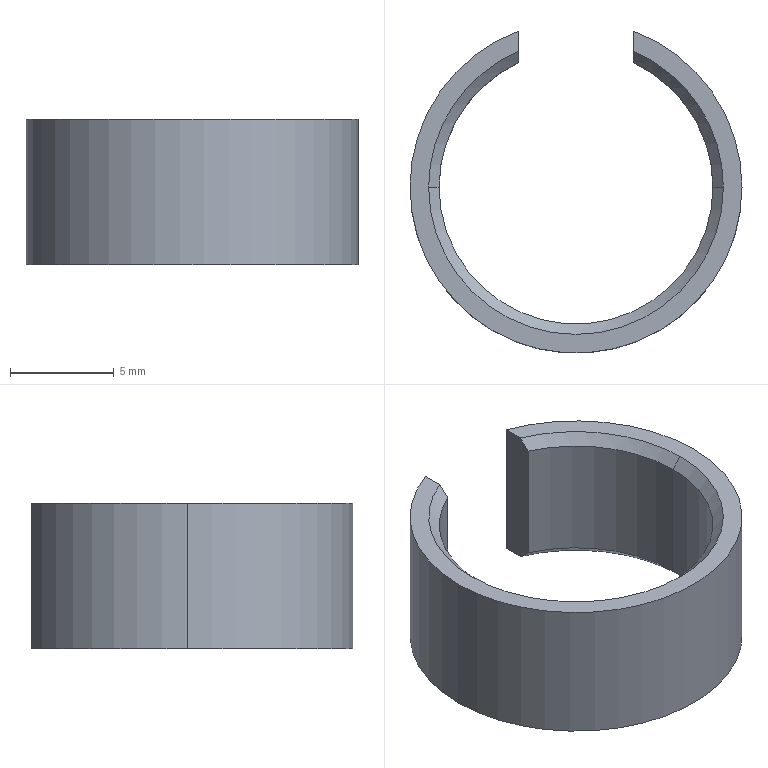Part | SolidWorks | features Chamfer 1, Extrusion 1, ICE 1 | 1 solid | 16 faces | box 16 x 15.512 x 7 mm | volume 385.007 mm3 | cone 6 | cylinder 6 | plane 4 | commonest cylinder face diameters 13.2 x3 16 x3
STEP:
#1=CARTESIAN_POINT('',(-6.6,0.,6.5));
#2=VERTEX_POINT('',#1);
#3=CARTESIAN_POINT('',(6.6,0.,6.5));
#4=VERTEX_POINT('',#3);
#5=CARTESIAN_POINT('',(0.,0.,6.5));
#6=DIRECTION('',(0.,0.,1.));
#7=DIRECTION('',(1.,0.,0.));
#8=AXIS2_PLACEMENT_3D('',#5,#6,#7);
#9=CIRCLE('',#8,6.6);
#10=EDGE_CURVE('',#2,#4,#9,.T.);
#11=ORIENTED_EDGE('',*,*,#10,.F.);
#12=CARTESIAN_POINT('',(-7.1,0.,7.));
#13=VERTEX_POINT('',#12);
#14=CARTESIAN_POINT('',(-6.6,0.,6.5));
#15=DIRECTION('',(-0.7071,0.,0.7071));
#16=VECTOR('',#15,1000.);
#17=LINE('',#14,#16);
#18=EDGE_CURVE('',#2,#13,#17,.T.);
#19=ORIENTED_EDGE('',*,*,#18,.T.);
#20=CARTESIAN_POINT('',(7.1,0.,7.));
#21=VERTEX_POINT('',#20);
#22=CARTESIAN_POINT('',(0.,0.,7.));
#23=DIRECTION('',(0.,0.,-1.));
#24=DIRECTION('',(1.,0.,0.));
#25=AXIS2_PLACEMENT_3D('',#22,#23,#24);
#26=CIRCLE('',#25,7.1);
#27=EDGE_CURVE('',#21,#13,#26,.T.);
#28=ORIENTED_EDGE('',*,*,#27,.F.);
#29=CARTESIAN_POINT('',(6.6,0.,6.5));
#30=DIRECTION('',(0.7071,0.,0.7071));
#31=VECTOR('',#30,1000.);
#32=LINE('',#29,#31);
#33=EDGE_CURVE('',#4,#21,#32,.T.);
#34=ORIENTED_EDGE('',*,*,#33,.F.);
#35=EDGE_LOOP('',(#11,#19,#28,#34));
#36=FACE_OUTER_BOUND('',#35,.T.);
#37=CARTESIAN_POINT('',(0.,0.,6.5));
#38=DIRECTION('',(0.,0.,1.));
#39=DIRECTION('',(1.,0.,0.));
#40=AXIS2_PLACEMENT_3D('',#37,#38,#39);
#41=CONICAL_SURFACE('',#40,6.6,0.7854);
#42=ADVANCED_FACE('',(#36),#41,.F.);
#43=CARTESIAN_POINT('',(2.75,6.,6.5));
#44=VERTEX_POINT('',#43);
#45=CARTESIAN_POINT('',(0.,0.,6.5));
#46=DIRECTION('',(0.,0.,1.));
#47=DIRECTION('',(1.,0.,0.));
#48=AXIS2_PLACEMENT_3D('',#45,#46,#47);
#49=CIRCLE('',#48,6.6);
#50=EDGE_CURVE('',#4,#44,#49,.T.);
#51=ORIENTED_EDGE('',*,*,#50,.F.);
#52=ORIENTED_EDGE('',*,*,#33,.T.);
#53=CARTESIAN_POINT('',(2.75,6.546,7.));
#54=VERTEX_POINT('',#53);
#55=CARTESIAN_POINT('',(0.,0.,7.));
#56=DIRECTION('',(0.,0.,-1.));
#57=DIRECTION('',(1.,0.,0.));
#58=AXIS2_PLACEMENT_3D('',#55,#56,#57);
#59=CIRCLE('',#58,7.1);
#60=EDGE_CURVE('',#54,#21,#59,.T.);
#61=ORIENTED_EDGE('',*,*,#60,.F.);
#62=CARTESIAN_POINT('',(2.75,6.,6.5));
#63=CARTESIAN_POINT('',(2.75,6.182,6.666));
#64=CARTESIAN_POINT('',(2.75,6.364,6.833));
#65=CARTESIAN_POINT('',(2.75,6.546,7.));
#66=B_SPLINE_CURVE_WITH_KNOTS('',3,(#62,#63,#64,#65),.UNSPECIFIED.,.F.,.F.,(4,4),(0.,0.0007404),.UNSPECIFIED.);
#67=EDGE_CURVE('',#44,#54,#66,.T.);
#68=ORIENTED_EDGE('',*,*,#67,.F.);
#69=EDGE_LOOP('',(#51,#52,#61,#68));
#70=FACE_OUTER_BOUND('',#69,.T.);
#71=CARTESIAN_POINT('',(0.,0.,6.5));
#72=DIRECTION('',(0.,0.,1.));
#73=DIRECTION('',(1.,0.,0.));
#74=AXIS2_PLACEMENT_3D('',#71,#72,#73);
#75=CONICAL_SURFACE('',#74,6.6,0.7854);
#76=ADVANCED_FACE('',(#70),#75,.F.);
#77=CARTESIAN_POINT('',(6.6,0.,0.5));
#78=VERTEX_POINT('',#77);
#79=CARTESIAN_POINT('',(-6.6,0.,0.5));
#80=VERTEX_POINT('',#79);
#81=CARTESIAN_POINT('',(0.,0.,0.5));
#82=DIRECTION('',(0.,0.,-1.));
#83=DIRECTION('',(1.,0.,0.));
#84=AXIS2_PLACEMENT_3D('',#81,#82,#83);
#85=CIRCLE('',#84,6.6);
#86=EDGE_CURVE('',#78,#80,#85,.T.);
#87=ORIENTED_EDGE('',*,*,#86,.F.);
#88=CARTESIAN_POINT('',(7.1,0.,0.));
#89=VERTEX_POINT('',#88);
#90=CARTESIAN_POINT('',(7.1,0.,0.));
#91=DIRECTION('',(0.7071,0.,-0.7071));
#92=VECTOR('',#91,1000.);
#93=LINE('',#90,#92);
#94=EDGE_CURVE('',#78,#89,#93,.T.);
#95=ORIENTED_EDGE('',*,*,#94,.T.);
#96=CARTESIAN_POINT('',(-7.1,0.,0.));
#97=VERTEX_POINT('',#96);
#98=CARTESIAN_POINT('',(0.,0.,0.));
#99=DIRECTION('',(0.,0.,1.));
#100=DIRECTION('',(1.,0.,0.));
#101=AXIS2_PLACEMENT_3D('',#98,#99,#100);
#102=CIRCLE('',#101,7.1);
#103=EDGE_CURVE('',#97,#89,#102,.T.);
#104=ORIENTED_EDGE('',*,*,#103,.F.);
#105=CARTESIAN_POINT('',(-7.1,0.,0.));
#106=DIRECTION('',(-0.7071,0.,-0.7071));
#107=VECTOR('',#106,1000.);
#108=LINE('',#105,#107);
#109=EDGE_CURVE('',#80,#97,#108,.T.);
#110=ORIENTED_EDGE('',*,*,#109,.F.);
#111=EDGE_LOOP('',(#87,#95,#104,#110));
#112=FACE_OUTER_BOUND('',#111,.T.);
#113=CARTESIAN_POINT('',(0.,0.,0.));
#114=DIRECTION('',(0.,0.,-1.));
#115=DIRECTION('',(-1.,0.,0.));
#116=AXIS2_PLACEMENT_3D('',#113,#114,#115);
#117=CONICAL_SURFACE('',#116,7.1,0.7854);
#118=ADVANCED_FACE('',(#112),#117,.F.);
#119=CARTESIAN_POINT('',(-2.75,6.,0.5));
#120=VERTEX_POINT('',#119);
#121=CARTESIAN_POINT('',(0.,0.,0.5));
#122=DIRECTION('',(0.,0.,-1.));
#123=DIRECTION('',(1.,0.,0.));
#124=AXIS2_PLACEMENT_3D('',#121,#122,#123);
#125=CIRCLE('',#124,6.6);
#126=EDGE_CURVE('',#80,#120,#125,.T.);
#127=ORIENTED_EDGE('',*,*,#126,.F.);
#128=ORIENTED_EDGE('',*,*,#109,.T.);
#129=CARTESIAN_POINT('',(-2.75,6.546,0.));
#130=VERTEX_POINT('',#129);
#131=CARTESIAN_POINT('',(0.,0.,0.));
#132=DIRECTION('',(0.,0.,1.));
#133=DIRECTION('',(1.,0.,0.));
#134=AXIS2_PLACEMENT_3D('',#131,#132,#133);
#135=CIRCLE('',#134,7.1);
#136=EDGE_CURVE('',#130,#97,#135,.T.);
#137=ORIENTED_EDGE('',*,*,#136,.F.);
#138=CARTESIAN_POINT('',(-2.75,6.,0.5));
#139=CARTESIAN_POINT('',(-2.75,6.182,0.334));
#140=CARTESIAN_POINT('',(-2.75,6.364,0.1673));
#141=CARTESIAN_POINT('',(-2.75,6.546,0.));
#142=B_SPLINE_CURVE_WITH_KNOTS('',3,(#138,#139,#140,#141),.UNSPECIFIED.,.F.,.F.,(4,4),(0.,0.0007404),.UNSPECIFIED.);
#143=EDGE_CURVE('',#120,#130,#142,.T.);
#144=ORIENTED_EDGE('',*,*,#143,.F.);
#145=EDGE_LOOP('',(#127,#128,#137,#144));
#146=FACE_OUTER_BOUND('',#145,.T.);
#147=CARTESIAN_POINT('',(0.,0.,0.));
#148=DIRECTION('',(0.,0.,-1.));
#149=DIRECTION('',(-1.,0.,0.));
#150=AXIS2_PLACEMENT_3D('',#147,#148,#149);
#151=CONICAL_SURFACE('',#150,7.1,0.7854);
#152=ADVANCED_FACE('',(#146),#151,.F.);
#153=ORIENTED_EDGE('',*,*,#10,.T.);
#154=CARTESIAN_POINT('',(6.6,0.,7.));
#155=DIRECTION('',(0.,0.,-1.));
#156=VECTOR('',#155,1000.);
#157=LINE('',#154,#156);
#158=EDGE_CURVE('',#4,#78,#157,.T.);
#159=ORIENTED_EDGE('',*,*,#158,.T.);
#160=ORIENTED_EDGE('',*,*,#86,.T.);
#161=CARTESIAN_POINT('',(-6.6,0.,7.));
#162=DIRECTION('',(0.,0.,-1.));
#163=VECTOR('',#162,1000.);
#164=LINE('',#161,#163);
#165=EDGE_CURVE('',#2,#80,#164,.T.);
#166=ORIENTED_EDGE('',*,*,#165,.F.);
#167=EDGE_LOOP('',(#153,#159,#160,#166));
#168=FACE_OUTER_BOUND('',#167,.T.);
#169=CARTESIAN_POINT('',(0.,0.,7.));
#170=DIRECTION('',(0.,0.,-1.));
#171=DIRECTION('',(-1.,0.,0.));
#172=AXIS2_PLACEMENT_3D('',#169,#170,#171);
#173=CYLINDRICAL_SURFACE('',#172,6.6);
#174=ADVANCED_FACE('',(#168),#173,.F.);
#175=CARTESIAN_POINT('',(-2.75,6.,6.5));
#176=VERTEX_POINT('',#175);
#177=CARTESIAN_POINT('',(0.,0.,6.5));
#178=DIRECTION('',(0.,0.,1.));
#179=DIRECTION('',(1.,0.,0.));
#180=AXIS2_PLACEMENT_3D('',#177,#178,#179);
#181=CIRCLE('',#180,6.6);
#182=EDGE_CURVE('',#176,#2,#181,.T.);
#183=ORIENTED_EDGE('',*,*,#182,.T.);
#184=ORIENTED_EDGE('',*,*,#165,.T.);
#185=ORIENTED_EDGE('',*,*,#126,.T.);
#186=CARTESIAN_POINT('',(-2.75,6.,7.));
#187=DIRECTION('',(0.,0.,-1.));
#188=VECTOR('',#187,1000.);
#189=LINE('',#186,#188);
#190=EDGE_CURVE('',#176,#120,#189,.T.);
#191=ORIENTED_EDGE('',*,*,#190,.F.);
#192=EDGE_LOOP('',(#183,#184,#185,#191));
#193=FACE_OUTER_BOUND('',#192,.T.);
#194=CARTESIAN_POINT('',(0.,0.,7.));
#195=DIRECTION('',(0.,0.,-1.));
#196=DIRECTION('',(-1.,0.,0.));
#197=AXIS2_PLACEMENT_3D('',#194,#195,#196);
#198=CYLINDRICAL_SURFACE('',#197,6.6);
#199=ADVANCED_FACE('',(#193),#198,.F.);
#200=CARTESIAN_POINT('',(8.,0.,7.));
#201=VERTEX_POINT('',#200);
#202=CARTESIAN_POINT('',(2.75,7.512,7.));
#203=VERTEX_POINT('',#202);
#204=CARTESIAN_POINT('',(0.,0.,7.));
#205=DIRECTION('',(0.,0.,1.));
#206=DIRECTION('',(1.,0.,0.));
#207=AXIS2_PLACEMENT_3D('',#204,#205,#206);
#208=CIRCLE('',#207,8.);
#209=EDGE_CURVE('',#201,#203,#208,.T.);
#210=ORIENTED_EDGE('',*,*,#209,.F.);
#211=CARTESIAN_POINT('',(8.,0.,0.));
#212=VERTEX_POINT('',#211);
#213=CARTESIAN_POINT('',(8.,0.,7.));
#214=DIRECTION('',(0.,0.,-1.));
#215=VECTOR('',#214,1000.);
#216=LINE('',#213,#215);
#217=EDGE_CURVE('',#201,#212,#216,.T.);
#218=ORIENTED_EDGE('',*,*,#217,.T.);
#219=CARTESIAN_POINT('',(2.75,7.512,0.));
#220=VERTEX_POINT('',#219);
#221=CARTESIAN_POINT('',(0.,0.,0.));
#222=DIRECTION('',(0.,0.,1.));
#223=DIRECTION('',(1.,0.,0.));
#224=AXIS2_PLACEMENT_3D('',#221,#222,#223);
#225=CIRCLE('',#224,8.);
#226=EDGE_CURVE('',#212,#220,#225,.T.);
#227=ORIENTED_EDGE('',*,*,#226,.T.);
#228=CARTESIAN_POINT('',(2.75,7.512,7.));
#229=DIRECTION('',(0.,0.,1.));
#230=VECTOR('',#229,1000.);
#231=LINE('',#228,#230);
#232=EDGE_CURVE('',#220,#203,#231,.T.);
#233=ORIENTED_EDGE('',*,*,#232,.T.);
#234=EDGE_LOOP('',(#210,#218,#227,#233));
#235=FACE_OUTER_BOUND('',#234,.T.);
#236=CARTESIAN_POINT('',(0.,0.,7.));
#237=DIRECTION('',(0.,0.,-1.));
#238=DIRECTION('',(-1.,0.,0.));
#239=AXIS2_PLACEMENT_3D('',#236,#237,#238);
#240=CYLINDRICAL_SURFACE('',#239,8.);
#241=ADVANCED_FACE('',(#235),#240,.T.);
#242=ORIENTED_EDGE('',*,*,#217,.F.);
#243=CARTESIAN_POINT('',(-8.,0.,7.));
#244=VERTEX_POINT('',#243);
#245=CARTESIAN_POINT('',(0.,0.,7.));
#246=DIRECTION('',(0.,0.,1.));
#247=DIRECTION('',(1.,0.,0.));
#248=AXIS2_PLACEMENT_3D('',#245,#246,#247);
#249=CIRCLE('',#248,8.);
#250=EDGE_CURVE('',#244,#201,#249,.T.);
#251=ORIENTED_EDGE('',*,*,#250,.F.);
#252=CARTESIAN_POINT('',(-8.,0.,0.));
#253=VERTEX_POINT('',#252);
#254=CARTESIAN_POINT('',(-8.,0.,7.));
#255=DIRECTION('',(0.,0.,-1.));
#256=VECTOR('',#255,1000.);
#257=LINE('',#254,#256);
#258=EDGE_CURVE('',#244,#253,#257,.T.);
#259=ORIENTED_EDGE('',*,*,#258,.T.);
#260=CARTESIAN_POINT('',(0.,0.,0.));
#261=DIRECTION('',(0.,0.,1.));
#262=DIRECTION('',(1.,0.,0.));
#263=AXIS2_PLACEMENT_3D('',#260,#261,#262);
#264=CIRCLE('',#263,8.);
#265=EDGE_CURVE('',#253,#212,#264,.T.);
#266=ORIENTED_EDGE('',*,*,#265,.T.);
#267=EDGE_LOOP('',(#242,#251,#259,#266));
#268=FACE_OUTER_BOUND('',#267,.T.);
#269=CARTESIAN_POINT('',(0.,0.,7.));
#270=DIRECTION('',(0.,0.,-1.));
#271=DIRECTION('',(-1.,0.,0.));
#272=AXIS2_PLACEMENT_3D('',#269,#270,#271);
#273=CYLINDRICAL_SURFACE('',#272,8.);
#274=ADVANCED_FACE('',(#268),#273,.T.);
#275=CARTESIAN_POINT('',(2.75,3.871,7.));
#276=DIRECTION('',(0.,1.,0.));
#277=VECTOR('',#276,1000.);
#278=LINE('',#275,#277);
#279=EDGE_CURVE('',#54,#203,#278,.T.);
#280=ORIENTED_EDGE('',*,*,#279,.F.);
#281=ORIENTED_EDGE('',*,*,#60,.T.);
#282=ORIENTED_EDGE('',*,*,#27,.T.);
#283=CARTESIAN_POINT('',(-2.75,6.546,7.));
#284=VERTEX_POINT('',#283);
#285=CARTESIAN_POINT('',(0.,0.,7.));
#286=DIRECTION('',(0.,0.,-1.));
#287=DIRECTION('',(1.,0.,0.));
#288=AXIS2_PLACEMENT_3D('',#285,#286,#287);
#289=CIRCLE('',#288,7.1);
#290=EDGE_CURVE('',#13,#284,#289,.T.);
#291=ORIENTED_EDGE('',*,*,#290,.T.);
#292=CARTESIAN_POINT('',(-2.75,7.512,7.));
#293=VERTEX_POINT('',#292);
#294=CARTESIAN_POINT('',(-2.75,3.871,7.));
#295=DIRECTION('',(0.,-1.,0.));
#296=VECTOR('',#295,1000.);
#297=LINE('',#294,#296);
#298=EDGE_CURVE('',#293,#284,#297,.T.);
#299=ORIENTED_EDGE('',*,*,#298,.F.);
#300=CARTESIAN_POINT('',(0.,0.,7.));
#301=DIRECTION('',(0.,0.,1.));
#302=DIRECTION('',(1.,0.,0.));
#303=AXIS2_PLACEMENT_3D('',#300,#301,#302);
#304=CIRCLE('',#303,8.);
#305=EDGE_CURVE('',#293,#244,#304,.T.);
#306=ORIENTED_EDGE('',*,*,#305,.T.);
#307=ORIENTED_EDGE('',*,*,#250,.T.);
#308=ORIENTED_EDGE('',*,*,#209,.T.);
#309=EDGE_LOOP('',(#280,#281,#282,#291,#299,#306,#307,#308));
#310=FACE_OUTER_BOUND('',#309,.T.);
#311=CARTESIAN_POINT('',(0.,0.,7.));
#312=DIRECTION('',(0.,0.,1.));
#313=DIRECTION('',(1.,0.,0.));
#314=AXIS2_PLACEMENT_3D('',#311,#312,#313);
#315=PLANE('',#314);
#316=ADVANCED_FACE('',(#310),#315,.T.);
#317=CARTESIAN_POINT('',(-2.75,7.512,0.));
#318=VERTEX_POINT('',#317);
#319=CARTESIAN_POINT('',(-2.75,3.871,0.));
#320=DIRECTION('',(0.,-1.,0.));
#321=VECTOR('',#320,1000.);
#322=LINE('',#319,#321);
#323=EDGE_CURVE('',#318,#130,#322,.T.);
#324=ORIENTED_EDGE('',*,*,#323,.T.);
#325=ORIENTED_EDGE('',*,*,#136,.T.);
#326=ORIENTED_EDGE('',*,*,#103,.T.);
#327=CARTESIAN_POINT('',(2.75,6.546,0.));
#328=VERTEX_POINT('',#327);
#329=CARTESIAN_POINT('',(0.,0.,0.));
#330=DIRECTION('',(0.,0.,1.));
#331=DIRECTION('',(1.,0.,0.));
#332=AXIS2_PLACEMENT_3D('',#329,#330,#331);
#333=CIRCLE('',#332,7.1);
#334=EDGE_CURVE('',#89,#328,#333,.T.);
#335=ORIENTED_EDGE('',*,*,#334,.T.);
#336=CARTESIAN_POINT('',(2.75,3.871,0.));
#337=DIRECTION('',(0.,1.,0.));
#338=VECTOR('',#337,1000.);
#339=LINE('',#336,#338);
#340=EDGE_CURVE('',#328,#220,#339,.T.);
#341=ORIENTED_EDGE('',*,*,#340,.T.);
#342=ORIENTED_EDGE('',*,*,#226,.F.);
#343=ORIENTED_EDGE('',*,*,#265,.F.);
#344=CARTESIAN_POINT('',(0.,0.,0.));
#345=DIRECTION('',(0.,0.,1.));
#346=DIRECTION('',(1.,0.,0.));
#347=AXIS2_PLACEMENT_3D('',#344,#345,#346);
#348=CIRCLE('',#347,8.);
#349=EDGE_CURVE('',#318,#253,#348,.T.);
#350=ORIENTED_EDGE('',*,*,#349,.F.);
#351=EDGE_LOOP('',(#324,#325,#326,#335,#341,#342,#343,#350));
#352=FACE_OUTER_BOUND('',#351,.T.);
#353=CARTESIAN_POINT('',(0.,0.,0.));
#354=DIRECTION('',(0.,0.,1.));
#355=DIRECTION('',(1.,0.,0.));
#356=AXIS2_PLACEMENT_3D('',#353,#354,#355);
#357=PLANE('',#356);
#358=ADVANCED_FACE('',(#352),#357,.F.);
#359=ORIENTED_EDGE('',*,*,#258,.F.);
#360=ORIENTED_EDGE('',*,*,#305,.F.);
#361=CARTESIAN_POINT('',(-2.75,7.512,7.));
#362=DIRECTION('',(0.,0.,-1.));
#363=VECTOR('',#362,1000.);
#364=LINE('',#361,#363);
#365=EDGE_CURVE('',#293,#318,#364,.T.);
#366=ORIENTED_EDGE('',*,*,#365,.T.);
#367=ORIENTED_EDGE('',*,*,#349,.T.);
#368=EDGE_LOOP('',(#359,#360,#366,#367));
#369=FACE_OUTER_BOUND('',#368,.T.);
#370=CARTESIAN_POINT('',(0.,0.,7.));
#371=DIRECTION('',(0.,0.,-1.));
#372=DIRECTION('',(-1.,0.,0.));
#373=AXIS2_PLACEMENT_3D('',#370,#371,#372);
#374=CYLINDRICAL_SURFACE('',#373,8.);
#375=ADVANCED_FACE('',(#369),#374,.T.);
#376=ORIENTED_EDGE('',*,*,#158,.F.);
#377=ORIENTED_EDGE('',*,*,#50,.T.);
#378=CARTESIAN_POINT('',(2.75,6.,0.5));
#379=VERTEX_POINT('',#378);
#380=CARTESIAN_POINT('',(2.75,6.,7.));
#381=DIRECTION('',(0.,0.,1.));
#382=VECTOR('',#381,1000.);
#383=LINE('',#380,#382);
#384=EDGE_CURVE('',#379,#44,#383,.T.);
#385=ORIENTED_EDGE('',*,*,#384,.F.);
#386=CARTESIAN_POINT('',(0.,0.,0.5));
#387=DIRECTION('',(0.,0.,-1.));
#388=DIRECTION('',(1.,0.,0.));
#389=AXIS2_PLACEMENT_3D('',#386,#387,#388);
#390=CIRCLE('',#389,6.6);
#391=EDGE_CURVE('',#379,#78,#390,.T.);
#392=ORIENTED_EDGE('',*,*,#391,.T.);
#393=EDGE_LOOP('',(#376,#377,#385,#392));
#394=FACE_OUTER_BOUND('',#393,.T.);
#395=CARTESIAN_POINT('',(0.,0.,7.));
#396=DIRECTION('',(0.,0.,-1.));
#397=DIRECTION('',(-1.,0.,0.));
#398=AXIS2_PLACEMENT_3D('',#395,#396,#397);
#399=CYLINDRICAL_SURFACE('',#398,6.6);
#400=ADVANCED_FACE('',(#394),#399,.F.);
#401=ORIENTED_EDGE('',*,*,#340,.F.);
#402=CARTESIAN_POINT('',(2.75,6.546,0.));
#403=CARTESIAN_POINT('',(2.75,6.364,0.1673));
#404=CARTESIAN_POINT('',(2.75,6.182,0.334));
#405=CARTESIAN_POINT('',(2.75,6.,0.5));
#406=B_SPLINE_CURVE_WITH_KNOTS('',3,(#402,#403,#404,#405),.UNSPECIFIED.,.F.,.F.,(4,4),(0.,0.0007404),.UNSPECIFIED.);
#407=EDGE_CURVE('',#328,#379,#406,.T.);
#408=ORIENTED_EDGE('',*,*,#407,.T.);
#409=ORIENTED_EDGE('',*,*,#384,.T.);
#410=ORIENTED_EDGE('',*,*,#67,.T.);
#411=ORIENTED_EDGE('',*,*,#279,.T.);
#412=ORIENTED_EDGE('',*,*,#232,.F.);
#413=EDGE_LOOP('',(#401,#408,#409,#410,#411,#412));
#414=FACE_OUTER_BOUND('',#413,.T.);
#415=CARTESIAN_POINT('',(2.75,3.871,0.));
#416=DIRECTION('',(1.,0.,0.));
#417=DIRECTION('',(0.,0.,-1.));
#418=AXIS2_PLACEMENT_3D('',#415,#416,#417);
#419=PLANE('',#418);
#420=ADVANCED_FACE('',(#414),#419,.F.);
#421=ORIENTED_EDGE('',*,*,#190,.T.);
#422=ORIENTED_EDGE('',*,*,#143,.T.);
#423=ORIENTED_EDGE('',*,*,#323,.F.);
#424=ORIENTED_EDGE('',*,*,#365,.F.);
#425=ORIENTED_EDGE('',*,*,#298,.T.);
#426=CARTESIAN_POINT('',(-2.75,6.546,7.));
#427=CARTESIAN_POINT('',(-2.75,6.364,6.833));
#428=CARTESIAN_POINT('',(-2.75,6.182,6.666));
#429=CARTESIAN_POINT('',(-2.75,6.,6.5));
#430=B_SPLINE_CURVE_WITH_KNOTS('',3,(#426,#427,#428,#429),.UNSPECIFIED.,.F.,.F.,(4,4),(0.,0.0007404),.UNSPECIFIED.);
#431=EDGE_CURVE('',#284,#176,#430,.T.);
#432=ORIENTED_EDGE('',*,*,#431,.T.);
#433=EDGE_LOOP('',(#421,#422,#423,#424,#425,#432));
#434=FACE_OUTER_BOUND('',#433,.T.);
#435=CARTESIAN_POINT('',(-2.75,3.871,0.));
#436=DIRECTION('',(-1.,0.,0.));
#437=DIRECTION('',(0.,0.,1.));
#438=AXIS2_PLACEMENT_3D('',#435,#436,#437);
#439=PLANE('',#438);
#440=ADVANCED_FACE('',(#434),#439,.F.);
#441=ORIENTED_EDGE('',*,*,#94,.F.);
#442=ORIENTED_EDGE('',*,*,#391,.F.);
#443=ORIENTED_EDGE('',*,*,#407,.F.);
#444=ORIENTED_EDGE('',*,*,#334,.F.);
#445=EDGE_LOOP('',(#441,#442,#443,#444));
#446=FACE_OUTER_BOUND('',#445,.T.);
#447=CARTESIAN_POINT('',(0.,0.,0.));
#448=DIRECTION('',(0.,0.,-1.));
#449=DIRECTION('',(-1.,0.,0.));
#450=AXIS2_PLACEMENT_3D('',#447,#448,#449);
#451=CONICAL_SURFACE('',#450,7.1,0.7854);
#452=ADVANCED_FACE('',(#446),#451,.F.);
#453=ORIENTED_EDGE('',*,*,#18,.F.);
#454=ORIENTED_EDGE('',*,*,#182,.F.);
#455=ORIENTED_EDGE('',*,*,#431,.F.);
#456=ORIENTED_EDGE('',*,*,#290,.F.);
#457=EDGE_LOOP('',(#453,#454,#455,#456));
#458=FACE_OUTER_BOUND('',#457,.T.);
#459=CARTESIAN_POINT('',(0.,0.,6.5));
#460=DIRECTION('',(0.,0.,1.));
#461=DIRECTION('',(1.,0.,0.));
#462=AXIS2_PLACEMENT_3D('',#459,#460,#461);
#463=CONICAL_SURFACE('',#462,6.6,0.7854);
#464=ADVANCED_FACE('',(#458),#463,.F.);
#465=CLOSED_SHELL('',(#42,#76,#118,#152,#174,#199,#241,#274,#316,#358,#375,#400,#420,#440,#452,#464));
#466=MANIFOLD_SOLID_BREP('',#465);
#467=CARTESIAN_POINT('',(0.,0.,0.));
#468=DIRECTION('',(0.,0.,1.));
#469=DIRECTION('',(1.,0.,0.));
#470=AXIS2_PLACEMENT_3D('',#467,#468,#469);
#471=(LENGTH_UNIT()NAMED_UNIT(*)SI_UNIT(.MILLI.,.METRE.));
#472=UNCERTAINTY_MEASURE_WITH_UNIT(LENGTH_MEASURE(0.00001),#471,'','');
#473=(NAMED_UNIT(*)PLANE_ANGLE_UNIT()SI_UNIT($,.RADIAN.));
#474=(NAMED_UNIT(*)SI_UNIT($,.STERADIAN.)SOLID_ANGLE_UNIT());
#475=(GEOMETRIC_REPRESENTATION_CONTEXT(3)GLOBAL_UNCERTAINTY_ASSIGNED_CONTEXT((#472))GLOBAL_UNIT_ASSIGNED_CONTEXT((#471,#473,#474))REPRESENTATION_CONTEXT('',''));
#476=ADVANCED_BREP_SHAPE_REPRESENTATION('',(#466,#470),#475);